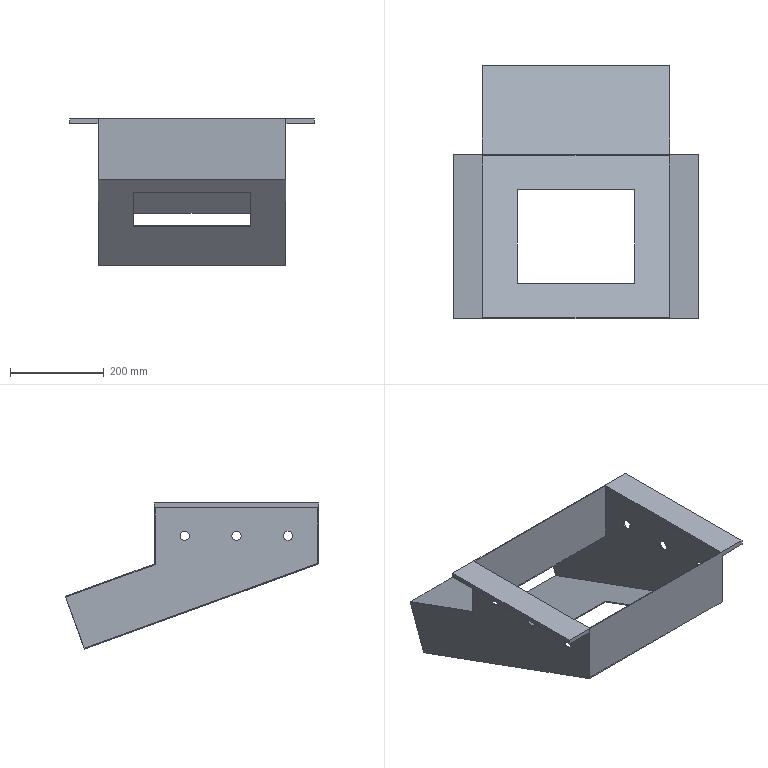Part | SolidWorks | features ICE 4, Extrusion 1, Shell 1 | 1 solid | 34 faces | box 520 x 538.979 x 311.271 mm | volume 1451807 mm3 | plane 22 | cylinder 12 | commonest cylinder face diameters 20 x12
STEP:
#1=CARTESIAN_POINT('',(198.,110.,50.));
#2=VERTEX_POINT('',#1);
#3=CARTESIAN_POINT('',(198.,110.,70.));
#4=VERTEX_POINT('',#3);
#5=CARTESIAN_POINT('',(198.,110.,60.));
#6=DIRECTION('',(-1.,0.,0.));
#7=DIRECTION('',(0.,0.,1.));
#8=AXIS2_PLACEMENT_3D('',#5,#6,#7);
#9=CIRCLE('',#8,10.);
#10=EDGE_CURVE('',#2,#4,#9,.T.);
#11=ORIENTED_EDGE('',*,*,#10,.T.);
#12=CARTESIAN_POINT('',(200.,110.,70.));
#13=VERTEX_POINT('',#12);
#14=CARTESIAN_POINT('',(-260.,110.,70.));
#15=DIRECTION('',(1.,0.,0.));
#16=VECTOR('',#15,1000.);
#17=LINE('',#14,#16);
#18=EDGE_CURVE('',#4,#13,#17,.T.);
#19=ORIENTED_EDGE('',*,*,#18,.T.);
#20=CARTESIAN_POINT('',(200.,110.,50.));
#21=VERTEX_POINT('',#20);
#22=CARTESIAN_POINT('',(200.,110.,60.));
#23=DIRECTION('',(1.,0.,0.));
#24=DIRECTION('',(0.,0.,-1.));
#25=AXIS2_PLACEMENT_3D('',#22,#23,#24);
#26=CIRCLE('',#25,10.);
#27=EDGE_CURVE('',#13,#21,#26,.T.);
#28=ORIENTED_EDGE('',*,*,#27,.T.);
#29=CARTESIAN_POINT('',(-260.,110.,50.));
#30=DIRECTION('',(1.,0.,0.));
#31=VECTOR('',#30,1000.);
#32=LINE('',#29,#31);
#33=EDGE_CURVE('',#2,#21,#32,.T.);
#34=ORIENTED_EDGE('',*,*,#33,.F.);
#35=EDGE_LOOP('',(#11,#19,#28,#34));
#36=FACE_OUTER_BOUND('',#35,.T.);
#37=CARTESIAN_POINT('',(-260.,110.,60.));
#38=DIRECTION('',(1.,0.,0.));
#39=DIRECTION('',(0.,0.,-1.));
#40=AXIS2_PLACEMENT_3D('',#37,#38,#39);
#41=CYLINDRICAL_SURFACE('',#40,10.);
#42=ADVANCED_FACE('',(#36),#41,.F.);
#43=CARTESIAN_POINT('',(198.,-110.,50.));
#44=VERTEX_POINT('',#43);
#45=CARTESIAN_POINT('',(198.,-110.,70.));
#46=VERTEX_POINT('',#45);
#47=CARTESIAN_POINT('',(198.,-110.,60.));
#48=DIRECTION('',(-1.,0.,0.));
#49=DIRECTION('',(0.,0.,1.));
#50=AXIS2_PLACEMENT_3D('',#47,#48,#49);
#51=CIRCLE('',#50,10.);
#52=EDGE_CURVE('',#44,#46,#51,.T.);
#53=ORIENTED_EDGE('',*,*,#52,.T.);
#54=CARTESIAN_POINT('',(200.,-110.,70.));
#55=VERTEX_POINT('',#54);
#56=CARTESIAN_POINT('',(-260.,-110.,70.));
#57=DIRECTION('',(1.,0.,0.));
#58=VECTOR('',#57,1000.);
#59=LINE('',#56,#58);
#60=EDGE_CURVE('',#46,#55,#59,.T.);
#61=ORIENTED_EDGE('',*,*,#60,.T.);
#62=CARTESIAN_POINT('',(200.,-110.,50.));
#63=VERTEX_POINT('',#62);
#64=CARTESIAN_POINT('',(200.,-110.,60.));
#65=DIRECTION('',(1.,0.,0.));
#66=DIRECTION('',(0.,0.,-1.));
#67=AXIS2_PLACEMENT_3D('',#64,#65,#66);
#68=CIRCLE('',#67,10.);
#69=EDGE_CURVE('',#55,#63,#68,.T.);
#70=ORIENTED_EDGE('',*,*,#69,.T.);
#71=CARTESIAN_POINT('',(-260.,-110.,50.));
#72=DIRECTION('',(1.,0.,0.));
#73=VECTOR('',#72,1000.);
#74=LINE('',#71,#73);
#75=EDGE_CURVE('',#44,#63,#74,.T.);
#76=ORIENTED_EDGE('',*,*,#75,.F.);
#77=EDGE_LOOP('',(#53,#61,#70,#76));
#78=FACE_OUTER_BOUND('',#77,.T.);
#79=CARTESIAN_POINT('',(-260.,-110.,60.));
#80=DIRECTION('',(1.,0.,0.));
#81=DIRECTION('',(0.,0.,-1.));
#82=AXIS2_PLACEMENT_3D('',#79,#80,#81);
#83=CYLINDRICAL_SURFACE('',#82,10.);
#84=ADVANCED_FACE('',(#78),#83,.F.);
#85=CARTESIAN_POINT('',(198.,0.,50.));
#86=VERTEX_POINT('',#85);
#87=CARTESIAN_POINT('',(198.,0.,70.));
#88=VERTEX_POINT('',#87);
#89=CARTESIAN_POINT('',(198.,0.,60.));
#90=DIRECTION('',(-1.,0.,0.));
#91=DIRECTION('',(0.,0.,1.));
#92=AXIS2_PLACEMENT_3D('',#89,#90,#91);
#93=CIRCLE('',#92,10.);
#94=EDGE_CURVE('',#86,#88,#93,.T.);
#95=ORIENTED_EDGE('',*,*,#94,.T.);
#96=CARTESIAN_POINT('',(200.,0.,70.));
#97=VERTEX_POINT('',#96);
#98=CARTESIAN_POINT('',(-260.,0.,70.));
#99=DIRECTION('',(1.,0.,0.));
#100=VECTOR('',#99,1000.);
#101=LINE('',#98,#100);
#102=EDGE_CURVE('',#88,#97,#101,.T.);
#103=ORIENTED_EDGE('',*,*,#102,.T.);
#104=CARTESIAN_POINT('',(200.,0.,50.));
#105=VERTEX_POINT('',#104);
#106=CARTESIAN_POINT('',(200.,0.,60.));
#107=DIRECTION('',(1.,0.,0.));
#108=DIRECTION('',(0.,0.,-1.));
#109=AXIS2_PLACEMENT_3D('',#106,#107,#108);
#110=CIRCLE('',#109,10.);
#111=EDGE_CURVE('',#97,#105,#110,.T.);
#112=ORIENTED_EDGE('',*,*,#111,.T.);
#113=CARTESIAN_POINT('',(-260.,0.,50.));
#114=DIRECTION('',(1.,0.,0.));
#115=VECTOR('',#114,1000.);
#116=LINE('',#113,#115);
#117=EDGE_CURVE('',#86,#105,#116,.T.);
#118=ORIENTED_EDGE('',*,*,#117,.F.);
#119=EDGE_LOOP('',(#95,#103,#112,#118));
#120=FACE_OUTER_BOUND('',#119,.T.);
#121=CARTESIAN_POINT('',(-260.,0.,60.));
#122=DIRECTION('',(1.,0.,0.));
#123=DIRECTION('',(0.,0.,-1.));
#124=AXIS2_PLACEMENT_3D('',#121,#122,#123);
#125=CYLINDRICAL_SURFACE('',#124,10.);
#126=ADVANCED_FACE('',(#120),#125,.F.);
#127=CARTESIAN_POINT('',(-200.,110.,70.));
#128=VERTEX_POINT('',#127);
#129=CARTESIAN_POINT('',(-200.,110.,50.));
#130=VERTEX_POINT('',#129);
#131=CARTESIAN_POINT('',(-200.,110.,60.));
#132=DIRECTION('',(1.,0.,0.));
#133=DIRECTION('',(0.,0.,-1.));
#134=AXIS2_PLACEMENT_3D('',#131,#132,#133);
#135=CIRCLE('',#134,10.);
#136=EDGE_CURVE('',#128,#130,#135,.T.);
#137=ORIENTED_EDGE('',*,*,#136,.F.);
#138=CARTESIAN_POINT('',(-198.,110.,70.));
#139=VERTEX_POINT('',#138);
#140=CARTESIAN_POINT('',(-260.,110.,70.));
#141=DIRECTION('',(1.,0.,0.));
#142=VECTOR('',#141,1000.);
#143=LINE('',#140,#142);
#144=EDGE_CURVE('',#128,#139,#143,.T.);
#145=ORIENTED_EDGE('',*,*,#144,.T.);
#146=CARTESIAN_POINT('',(-198.,110.,50.));
#147=VERTEX_POINT('',#146);
#148=CARTESIAN_POINT('',(-198.,110.,60.));
#149=DIRECTION('',(1.,0.,0.));
#150=DIRECTION('',(0.,0.,-1.));
#151=AXIS2_PLACEMENT_3D('',#148,#149,#150);
#152=CIRCLE('',#151,10.);
#153=EDGE_CURVE('',#139,#147,#152,.T.);
#154=ORIENTED_EDGE('',*,*,#153,.T.);
#155=CARTESIAN_POINT('',(-260.,110.,50.));
#156=DIRECTION('',(1.,0.,0.));
#157=VECTOR('',#156,1000.);
#158=LINE('',#155,#157);
#159=EDGE_CURVE('',#130,#147,#158,.T.);
#160=ORIENTED_EDGE('',*,*,#159,.F.);
#161=EDGE_LOOP('',(#137,#145,#154,#160));
#162=FACE_OUTER_BOUND('',#161,.T.);
#163=CARTESIAN_POINT('',(-260.,110.,60.));
#164=DIRECTION('',(1.,0.,0.));
#165=DIRECTION('',(0.,0.,-1.));
#166=AXIS2_PLACEMENT_3D('',#163,#164,#165);
#167=CYLINDRICAL_SURFACE('',#166,10.);
#168=ADVANCED_FACE('',(#162),#167,.F.);
#169=CARTESIAN_POINT('',(-200.,-110.,70.));
#170=VERTEX_POINT('',#169);
#171=CARTESIAN_POINT('',(-200.,-110.,50.));
#172=VERTEX_POINT('',#171);
#173=CARTESIAN_POINT('',(-200.,-110.,60.));
#174=DIRECTION('',(1.,0.,0.));
#175=DIRECTION('',(0.,0.,-1.));
#176=AXIS2_PLACEMENT_3D('',#173,#174,#175);
#177=CIRCLE('',#176,10.);
#178=EDGE_CURVE('',#170,#172,#177,.T.);
#179=ORIENTED_EDGE('',*,*,#178,.F.);
#180=CARTESIAN_POINT('',(-198.,-110.,70.));
#181=VERTEX_POINT('',#180);
#182=CARTESIAN_POINT('',(-260.,-110.,70.));
#183=DIRECTION('',(1.,0.,0.));
#184=VECTOR('',#183,1000.);
#185=LINE('',#182,#184);
#186=EDGE_CURVE('',#170,#181,#185,.T.);
#187=ORIENTED_EDGE('',*,*,#186,.T.);
#188=CARTESIAN_POINT('',(-198.,-110.,50.));
#189=VERTEX_POINT('',#188);
#190=CARTESIAN_POINT('',(-198.,-110.,60.));
#191=DIRECTION('',(1.,0.,0.));
#192=DIRECTION('',(0.,0.,-1.));
#193=AXIS2_PLACEMENT_3D('',#190,#191,#192);
#194=CIRCLE('',#193,10.);
#195=EDGE_CURVE('',#181,#189,#194,.T.);
#196=ORIENTED_EDGE('',*,*,#195,.T.);
#197=CARTESIAN_POINT('',(-260.,-110.,50.));
#198=DIRECTION('',(1.,0.,0.));
#199=VECTOR('',#198,1000.);
#200=LINE('',#197,#199);
#201=EDGE_CURVE('',#172,#189,#200,.T.);
#202=ORIENTED_EDGE('',*,*,#201,.F.);
#203=EDGE_LOOP('',(#179,#187,#196,#202));
#204=FACE_OUTER_BOUND('',#203,.T.);
#205=CARTESIAN_POINT('',(-260.,-110.,60.));
#206=DIRECTION('',(1.,0.,0.));
#207=DIRECTION('',(0.,0.,-1.));
#208=AXIS2_PLACEMENT_3D('',#205,#206,#207);
#209=CYLINDRICAL_SURFACE('',#208,10.);
#210=ADVANCED_FACE('',(#204),#209,.F.);
#211=CARTESIAN_POINT('',(-200.,0.,70.));
#212=VERTEX_POINT('',#211);
#213=CARTESIAN_POINT('',(-200.,0.,50.));
#214=VERTEX_POINT('',#213);
#215=CARTESIAN_POINT('',(-200.,0.,60.));
#216=DIRECTION('',(1.,0.,0.));
#217=DIRECTION('',(0.,0.,-1.));
#218=AXIS2_PLACEMENT_3D('',#215,#216,#217);
#219=CIRCLE('',#218,10.);
#220=EDGE_CURVE('',#212,#214,#219,.T.);
#221=ORIENTED_EDGE('',*,*,#220,.F.);
#222=CARTESIAN_POINT('',(-198.,0.,70.));
#223=VERTEX_POINT('',#222);
#224=CARTESIAN_POINT('',(-260.,0.,70.));
#225=DIRECTION('',(1.,0.,0.));
#226=VECTOR('',#225,1000.);
#227=LINE('',#224,#226);
#228=EDGE_CURVE('',#212,#223,#227,.T.);
#229=ORIENTED_EDGE('',*,*,#228,.T.);
#230=CARTESIAN_POINT('',(-198.,0.,50.));
#231=VERTEX_POINT('',#230);
#232=CARTESIAN_POINT('',(-198.,0.,60.));
#233=DIRECTION('',(1.,0.,0.));
#234=DIRECTION('',(0.,0.,-1.));
#235=AXIS2_PLACEMENT_3D('',#232,#233,#234);
#236=CIRCLE('',#235,10.);
#237=EDGE_CURVE('',#223,#231,#236,.T.);
#238=ORIENTED_EDGE('',*,*,#237,.T.);
#239=CARTESIAN_POINT('',(-260.,0.,50.));
#240=DIRECTION('',(1.,0.,0.));
#241=VECTOR('',#240,1000.);
#242=LINE('',#239,#241);
#243=EDGE_CURVE('',#214,#231,#242,.T.);
#244=ORIENTED_EDGE('',*,*,#243,.F.);
#245=EDGE_LOOP('',(#221,#229,#238,#244));
#246=FACE_OUTER_BOUND('',#245,.T.);
#247=CARTESIAN_POINT('',(-260.,0.,60.));
#248=DIRECTION('',(1.,0.,0.));
#249=DIRECTION('',(0.,0.,-1.));
#250=AXIS2_PLACEMENT_3D('',#247,#248,#249);
#251=CYLINDRICAL_SURFACE('',#250,10.);
#252=ADVANCED_FACE('',(#246),#251,.F.);
#253=CARTESIAN_POINT('',(-260.,-175.,130.));
#254=VERTEX_POINT('',#253);
#255=CARTESIAN_POINT('',(260.,-175.,130.));
#256=VERTEX_POINT('',#255);
#257=CARTESIAN_POINT('',(-200.,-175.,130.));
#258=DIRECTION('',(1.,0.,0.));
#259=VECTOR('',#258,1000.);
#260=LINE('',#257,#259);
#261=EDGE_CURVE('',#254,#256,#260,.T.);
#262=ORIENTED_EDGE('',*,*,#261,.T.);
#263=CARTESIAN_POINT('',(260.,175.,130.));
#264=VERTEX_POINT('',#263);
#265=CARTESIAN_POINT('',(260.,175.,130.));
#266=DIRECTION('',(0.,1.,0.));
#267=VECTOR('',#266,1000.);
#268=LINE('',#265,#267);
#269=EDGE_CURVE('',#256,#264,#268,.T.);
#270=ORIENTED_EDGE('',*,*,#269,.T.);
#271=CARTESIAN_POINT('',(-260.,175.,130.));
#272=VERTEX_POINT('',#271);
#273=CARTESIAN_POINT('',(-200.,175.,130.));
#274=DIRECTION('',(-1.,0.,0.));
#275=VECTOR('',#274,1000.);
#276=LINE('',#273,#275);
#277=EDGE_CURVE('',#264,#272,#276,.T.);
#278=ORIENTED_EDGE('',*,*,#277,.T.);
#279=CARTESIAN_POINT('',(-260.,175.,130.));
#280=DIRECTION('',(0.,-1.,0.));
#281=VECTOR('',#280,1000.);
#282=LINE('',#279,#281);
#283=EDGE_CURVE('',#272,#254,#282,.T.);
#284=ORIENTED_EDGE('',*,*,#283,.T.);
#285=EDGE_LOOP('',(#262,#270,#278,#284));
#286=FACE_OUTER_BOUND('',#285,.T.);
#287=CARTESIAN_POINT('',(198.,-173.,130.));
#288=VERTEX_POINT('',#287);
#289=CARTESIAN_POINT('',(198.,173.,130.));
#290=VERTEX_POINT('',#289);
#291=CARTESIAN_POINT('',(198.,0.,130.));
#292=DIRECTION('',(0.,1.,0.));
#293=VECTOR('',#292,1000.);
#294=LINE('',#291,#293);
#295=EDGE_CURVE('',#288,#290,#294,.T.);
#296=ORIENTED_EDGE('',*,*,#295,.F.);
#297=CARTESIAN_POINT('',(-198.,-173.,130.));
#298=VERTEX_POINT('',#297);
#299=CARTESIAN_POINT('',(0.,-173.,130.));
#300=DIRECTION('',(1.,0.,0.));
#301=VECTOR('',#300,1000.);
#302=LINE('',#299,#301);
#303=EDGE_CURVE('',#298,#288,#302,.T.);
#304=ORIENTED_EDGE('',*,*,#303,.F.);
#305=CARTESIAN_POINT('',(-198.,173.,130.));
#306=VERTEX_POINT('',#305);
#307=CARTESIAN_POINT('',(-198.,0.,130.));
#308=DIRECTION('',(0.,-1.,0.));
#309=VECTOR('',#308,1000.);
#310=LINE('',#307,#309);
#311=EDGE_CURVE('',#306,#298,#310,.T.);
#312=ORIENTED_EDGE('',*,*,#311,.F.);
#313=CARTESIAN_POINT('',(0.,173.,130.));
#314=DIRECTION('',(-1.,0.,0.));
#315=VECTOR('',#314,1000.);
#316=LINE('',#313,#315);
#317=EDGE_CURVE('',#290,#306,#316,.T.);
#318=ORIENTED_EDGE('',*,*,#317,.F.);
#319=EDGE_LOOP('',(#296,#304,#312,#318));
#320=FACE_BOUND('',#319,.T.);
#321=CARTESIAN_POINT('',(0.,0.,130.));
#322=DIRECTION('',(0.,0.,-1.));
#323=DIRECTION('',(-1.,0.,0.));
#324=AXIS2_PLACEMENT_3D('',#321,#322,#323);
#325=PLANE('',#324);
#326=ADVANCED_FACE('',(#286,#320),#325,.F.);
#327=CARTESIAN_POINT('',(200.,323.037,-181.271));
#328=VERTEX_POINT('',#327);
#329=CARTESIAN_POINT('',(200.,363.979,-68.783));
#330=VERTEX_POINT('',#329);
#331=CARTESIAN_POINT('',(200.,363.979,-68.783));
#332=DIRECTION('',(0.,0.342,0.9397));
#333=VECTOR('',#332,1000.);
#334=LINE('',#331,#333);
#335=EDGE_CURVE('',#328,#330,#334,.T.);
#336=ORIENTED_EDGE('',*,*,#335,.F.);
#337=CARTESIAN_POINT('',(-200.,323.037,-181.271));
#338=VERTEX_POINT('',#337);
#339=CARTESIAN_POINT('',(768.646,323.037,-181.271));
#340=DIRECTION('',(-1.,0.,0.));
#341=VECTOR('',#340,1000.);
#342=LINE('',#339,#341);
#343=EDGE_CURVE('',#328,#338,#342,.T.);
#344=ORIENTED_EDGE('',*,*,#343,.T.);
#345=CARTESIAN_POINT('',(-200.,363.979,-68.783));
#346=VERTEX_POINT('',#345);
#347=CARTESIAN_POINT('',(-200.,363.979,-68.783));
#348=DIRECTION('',(0.,-0.342,-0.9397));
#349=VECTOR('',#348,1000.);
#350=LINE('',#347,#349);
#351=EDGE_CURVE('',#346,#338,#350,.T.);
#352=ORIENTED_EDGE('',*,*,#351,.F.);
#353=CARTESIAN_POINT('',(768.646,363.979,-68.783));
#354=DIRECTION('',(-1.,0.,0.));
#355=VECTOR('',#354,1000.);
#356=LINE('',#353,#355);
#357=EDGE_CURVE('',#330,#346,#356,.T.);
#358=ORIENTED_EDGE('',*,*,#357,.F.);
#359=EDGE_LOOP('',(#336,#344,#352,#358));
#360=FACE_OUTER_BOUND('',#359,.T.);
#361=CARTESIAN_POINT('',(198.,323.721,-179.391));
#362=VERTEX_POINT('',#361);
#363=CARTESIAN_POINT('',(-198.,323.721,-179.391));
#364=VERTEX_POINT('',#363);
#365=CARTESIAN_POINT('',(768.646,323.721,-179.391));
#366=DIRECTION('',(-1.,0.,0.));
#367=VECTOR('',#366,1000.);
#368=LINE('',#365,#367);
#369=EDGE_CURVE('',#362,#364,#368,.T.);
#370=ORIENTED_EDGE('',*,*,#369,.F.);
#371=CARTESIAN_POINT('',(198.,363.295,-70.662));
#372=VERTEX_POINT('',#371);
#373=CARTESIAN_POINT('',(198.,363.979,-68.783));
#374=DIRECTION('',(0.,0.342,0.9397));
#375=VECTOR('',#374,1000.);
#376=LINE('',#373,#375);
#377=EDGE_CURVE('',#362,#372,#376,.T.);
#378=ORIENTED_EDGE('',*,*,#377,.T.);
#379=CARTESIAN_POINT('',(-198.,363.295,-70.662));
#380=VERTEX_POINT('',#379);
#381=CARTESIAN_POINT('',(768.646,363.295,-70.662));
#382=DIRECTION('',(-1.,0.,0.));
#383=VECTOR('',#382,1000.);
#384=LINE('',#381,#383);
#385=EDGE_CURVE('',#372,#380,#384,.T.);
#386=ORIENTED_EDGE('',*,*,#385,.T.);
#387=CARTESIAN_POINT('',(-198.,363.979,-68.783));
#388=DIRECTION('',(0.,-0.342,-0.9397));
#389=VECTOR('',#388,1000.);
#390=LINE('',#387,#389);
#391=EDGE_CURVE('',#380,#364,#390,.T.);
#392=ORIENTED_EDGE('',*,*,#391,.T.);
#393=EDGE_LOOP('',(#370,#378,#386,#392));
#394=FACE_BOUND('',#393,.T.);
#395=CARTESIAN_POINT('',(768.646,363.979,-68.783));
#396=DIRECTION('',(0.,0.9397,-0.342));
#397=DIRECTION('',(0.,0.342,0.9397));
#398=AXIS2_PLACEMENT_3D('',#395,#396,#397);
#399=PLANE('',#398);
#400=ADVANCED_FACE('',(#360,#394),#399,.T.);
#401=CARTESIAN_POINT('',(200.,110.,60.));
#402=DIRECTION('',(1.,0.,0.));
#403=DIRECTION('',(0.,0.,-1.));
#404=AXIS2_PLACEMENT_3D('',#401,#402,#403);
#405=CIRCLE('',#404,10.);
#406=EDGE_CURVE('',#21,#13,#405,.T.);
#407=ORIENTED_EDGE('',*,*,#406,.F.);
#408=ORIENTED_EDGE('',*,*,#27,.F.);
#409=EDGE_LOOP('',(#407,#408));
#410=FACE_BOUND('',#409,.T.);
#411=CARTESIAN_POINT('',(200.,-110.,60.));
#412=DIRECTION('',(1.,0.,0.));
#413=DIRECTION('',(0.,0.,-1.));
#414=AXIS2_PLACEMENT_3D('',#411,#412,#413);
#415=CIRCLE('',#414,10.);
#416=EDGE_CURVE('',#63,#55,#415,.T.);
#417=ORIENTED_EDGE('',*,*,#416,.F.);
#418=ORIENTED_EDGE('',*,*,#69,.F.);
#419=EDGE_LOOP('',(#417,#418));
#420=FACE_BOUND('',#419,.T.);
#421=CARTESIAN_POINT('',(200.,0.,60.));
#422=DIRECTION('',(1.,0.,0.));
#423=DIRECTION('',(0.,0.,-1.));
#424=AXIS2_PLACEMENT_3D('',#421,#422,#423);
#425=CIRCLE('',#424,10.);
#426=EDGE_CURVE('',#105,#97,#425,.T.);
#427=ORIENTED_EDGE('',*,*,#426,.F.);
#428=ORIENTED_EDGE('',*,*,#111,.F.);
#429=EDGE_LOOP('',(#427,#428));
#430=FACE_BOUND('',#429,.T.);
#431=CARTESIAN_POINT('',(200.,175.,120.));
#432=VERTEX_POINT('',#431);
#433=CARTESIAN_POINT('',(200.,175.,0.));
#434=VERTEX_POINT('',#433);
#435=CARTESIAN_POINT('',(200.,175.,130.));
#436=DIRECTION('',(0.,0.,-1.));
#437=VECTOR('',#436,1000.);
#438=LINE('',#435,#437);
#439=EDGE_CURVE('',#432,#434,#438,.T.);
#440=ORIENTED_EDGE('',*,*,#439,.F.);
#441=CARTESIAN_POINT('',(200.,-175.,120.));
#442=VERTEX_POINT('',#441);
#443=CARTESIAN_POINT('',(200.,175.,120.));
#444=DIRECTION('',(0.,-1.,0.));
#445=VECTOR('',#444,1000.);
#446=LINE('',#443,#445);
#447=EDGE_CURVE('',#432,#442,#446,.T.);
#448=ORIENTED_EDGE('',*,*,#447,.T.);
#449=CARTESIAN_POINT('',(200.,-175.,0.));
#450=VERTEX_POINT('',#449);
#451=CARTESIAN_POINT('',(200.,-175.,130.));
#452=DIRECTION('',(0.,0.,-1.));
#453=VECTOR('',#452,1000.);
#454=LINE('',#451,#453);
#455=EDGE_CURVE('',#442,#450,#454,.T.);
#456=ORIENTED_EDGE('',*,*,#455,.T.);
#457=CARTESIAN_POINT('',(200.,323.037,-181.271));
#458=DIRECTION('',(0.,0.9397,-0.342));
#459=VECTOR('',#458,1000.);
#460=LINE('',#457,#459);
#461=EDGE_CURVE('',#450,#328,#460,.T.);
#462=ORIENTED_EDGE('',*,*,#461,.T.);
#463=ORIENTED_EDGE('',*,*,#335,.T.);
#464=CARTESIAN_POINT('',(200.,175.,0.));
#465=DIRECTION('',(0.,-0.9397,0.342));
#466=VECTOR('',#465,1000.);
#467=LINE('',#464,#466);
#468=EDGE_CURVE('',#330,#434,#467,.T.);
#469=ORIENTED_EDGE('',*,*,#468,.T.);
#470=EDGE_LOOP('',(#440,#448,#456,#462,#463,#469));
#471=FACE_OUTER_BOUND('',#470,.T.);
#472=CARTESIAN_POINT('',(200.,-175.,130.));
#473=DIRECTION('',(-1.,0.,0.));
#474=DIRECTION('',(0.,0.,1.));
#475=AXIS2_PLACEMENT_3D('',#472,#473,#474);
#476=PLANE('',#475);
#477=ADVANCED_FACE('',(#410,#420,#430,#471),#476,.F.);
#478=CARTESIAN_POINT('',(-200.,175.,0.));
#479=VERTEX_POINT('',#478);
#480=CARTESIAN_POINT('',(-200.,175.,0.));
#481=DIRECTION('',(-1.,0.,0.));
#482=VECTOR('',#481,1000.);
#483=LINE('',#480,#482);
#484=EDGE_CURVE('',#434,#479,#483,.T.);
#485=ORIENTED_EDGE('',*,*,#484,.T.);
#486=CARTESIAN_POINT('',(-200.,175.,120.));
#487=VERTEX_POINT('',#486);
#488=CARTESIAN_POINT('',(-200.,175.,130.));
#489=DIRECTION('',(0.,0.,-1.));
#490=VECTOR('',#489,1000.);
#491=LINE('',#488,#490);
#492=EDGE_CURVE('',#487,#479,#491,.T.);
#493=ORIENTED_EDGE('',*,*,#492,.F.);
#494=CARTESIAN_POINT('',(-260.,175.,120.));
#495=VERTEX_POINT('',#494);
#496=CARTESIAN_POINT('',(-200.,175.,120.));
#497=DIRECTION('',(-1.,0.,0.));
#498=VECTOR('',#497,1000.);
#499=LINE('',#496,#498);
#500=EDGE_CURVE('',#487,#495,#499,.T.);
#501=ORIENTED_EDGE('',*,*,#500,.T.);
#502=CARTESIAN_POINT('',(-260.,175.,120.));
#503=DIRECTION('',(0.,0.,1.));
#504=VECTOR('',#503,1000.);
#505=LINE('',#502,#504);
#506=EDGE_CURVE('',#495,#272,#505,.T.);
#507=ORIENTED_EDGE('',*,*,#506,.T.);
#508=ORIENTED_EDGE('',*,*,#277,.F.);
#509=CARTESIAN_POINT('',(260.,175.,120.));
#510=VERTEX_POINT('',#509);
#511=CARTESIAN_POINT('',(260.,175.,120.));
#512=DIRECTION('',(0.,0.,1.));
#513=VECTOR('',#512,1000.);
#514=LINE('',#511,#513);
#515=EDGE_CURVE('',#510,#264,#514,.T.);
#516=ORIENTED_EDGE('',*,*,#515,.F.);
#517=CARTESIAN_POINT('',(200.,175.,120.));
#518=DIRECTION('',(-1.,0.,0.));
#519=VECTOR('',#518,1000.);
#520=LINE('',#517,#519);
#521=EDGE_CURVE('',#510,#432,#520,.T.);
#522=ORIENTED_EDGE('',*,*,#521,.T.);
#523=ORIENTED_EDGE('',*,*,#439,.T.);
#524=EDGE_LOOP('',(#485,#493,#501,#507,#508,#516,#522,#523));
#525=FACE_OUTER_BOUND('',#524,.T.);
#526=CARTESIAN_POINT('',(-200.,175.,130.));
#527=DIRECTION('',(0.,-1.,0.));
#528=DIRECTION('',(0.,0.,-1.));
#529=AXIS2_PLACEMENT_3D('',#526,#527,#528);
#530=PLANE('',#529);
#531=ADVANCED_FACE('',(#525),#530,.F.);
#532=CARTESIAN_POINT('',(-200.,110.,60.));
#533=DIRECTION('',(1.,0.,0.));
#534=DIRECTION('',(0.,0.,-1.));
#535=AXIS2_PLACEMENT_3D('',#532,#533,#534);
#536=CIRCLE('',#535,10.);
#537=EDGE_CURVE('',#130,#128,#536,.T.);
#538=ORIENTED_EDGE('',*,*,#537,.T.);
#539=ORIENTED_EDGE('',*,*,#136,.T.);
#540=EDGE_LOOP('',(#538,#539));
#541=FACE_BOUND('',#540,.T.);
#542=CARTESIAN_POINT('',(-200.,-110.,60.));
#543=DIRECTION('',(1.,0.,0.));
#544=DIRECTION('',(0.,0.,-1.));
#545=AXIS2_PLACEMENT_3D('',#542,#543,#544);
#546=CIRCLE('',#545,10.);
#547=EDGE_CURVE('',#172,#170,#546,.T.);
#548=ORIENTED_EDGE('',*,*,#547,.T.);
#549=ORIENTED_EDGE('',*,*,#178,.T.);
#550=EDGE_LOOP('',(#548,#549));
#551=FACE_BOUND('',#550,.T.);
#552=CARTESIAN_POINT('',(-200.,0.,60.));
#553=DIRECTION('',(1.,0.,0.));
#554=DIRECTION('',(0.,0.,-1.));
#555=AXIS2_PLACEMENT_3D('',#552,#553,#554);
#556=CIRCLE('',#555,10.);
#557=EDGE_CURVE('',#214,#212,#556,.T.);
#558=ORIENTED_EDGE('',*,*,#557,.T.);
#559=ORIENTED_EDGE('',*,*,#220,.T.);
#560=EDGE_LOOP('',(#558,#559));
#561=FACE_BOUND('',#560,.T.);
#562=CARTESIAN_POINT('',(-200.,-175.,120.));
#563=VERTEX_POINT('',#562);
#564=CARTESIAN_POINT('',(-200.,-175.,0.));
#565=VERTEX_POINT('',#564);
#566=CARTESIAN_POINT('',(-200.,-175.,130.));
#567=DIRECTION('',(0.,0.,-1.));
#568=VECTOR('',#567,1000.);
#569=LINE('',#566,#568);
#570=EDGE_CURVE('',#563,#565,#569,.T.);
#571=ORIENTED_EDGE('',*,*,#570,.F.);
#572=CARTESIAN_POINT('',(-200.,175.,120.));
#573=DIRECTION('',(0.,1.,0.));
#574=VECTOR('',#573,1000.);
#575=LINE('',#572,#574);
#576=EDGE_CURVE('',#563,#487,#575,.T.);
#577=ORIENTED_EDGE('',*,*,#576,.T.);
#578=ORIENTED_EDGE('',*,*,#492,.T.);
#579=CARTESIAN_POINT('',(-200.,175.,0.));
#580=DIRECTION('',(0.,0.9397,-0.342));
#581=VECTOR('',#580,1000.);
#582=LINE('',#579,#581);
#583=EDGE_CURVE('',#479,#346,#582,.T.);
#584=ORIENTED_EDGE('',*,*,#583,.T.);
#585=ORIENTED_EDGE('',*,*,#351,.T.);
#586=CARTESIAN_POINT('',(-200.,323.037,-181.271));
#587=DIRECTION('',(0.,-0.9397,0.342));
#588=VECTOR('',#587,1000.);
#589=LINE('',#586,#588);
#590=EDGE_CURVE('',#338,#565,#589,.T.);
#591=ORIENTED_EDGE('',*,*,#590,.T.);
#592=EDGE_LOOP('',(#571,#577,#578,#584,#585,#591));
#593=FACE_OUTER_BOUND('',#592,.T.);
#594=CARTESIAN_POINT('',(-200.,-175.,130.));
#595=DIRECTION('',(1.,0.,0.));
#596=DIRECTION('',(0.,0.,-1.));
#597=AXIS2_PLACEMENT_3D('',#594,#595,#596);
#598=PLANE('',#597);
#599=ADVANCED_FACE('',(#541,#551,#561,#593),#598,.F.);
#600=CARTESIAN_POINT('',(-200.,-175.,0.));
#601=DIRECTION('',(1.,0.,0.));
#602=VECTOR('',#601,1000.);
#603=LINE('',#600,#602);
#604=EDGE_CURVE('',#565,#450,#603,.T.);
#605=ORIENTED_EDGE('',*,*,#604,.T.);
#606=ORIENTED_EDGE('',*,*,#455,.F.);
#607=CARTESIAN_POINT('',(260.,-175.,120.));
#608=VERTEX_POINT('',#607);
#609=CARTESIAN_POINT('',(200.,-175.,120.));
#610=DIRECTION('',(1.,0.,0.));
#611=VECTOR('',#610,1000.);
#612=LINE('',#609,#611);
#613=EDGE_CURVE('',#442,#608,#612,.T.);
#614=ORIENTED_EDGE('',*,*,#613,.T.);
#615=CARTESIAN_POINT('',(260.,-175.,120.));
#616=DIRECTION('',(0.,0.,1.));
#617=VECTOR('',#616,1000.);
#618=LINE('',#615,#617);
#619=EDGE_CURVE('',#608,#256,#618,.T.);
#620=ORIENTED_EDGE('',*,*,#619,.T.);
#621=ORIENTED_EDGE('',*,*,#261,.F.);
#622=CARTESIAN_POINT('',(-260.,-175.,120.));
#623=VERTEX_POINT('',#622);
#624=CARTESIAN_POINT('',(-260.,-175.,120.));
#625=DIRECTION('',(0.,0.,1.));
#626=VECTOR('',#625,1000.);
#627=LINE('',#624,#626);
#628=EDGE_CURVE('',#623,#254,#627,.T.);
#629=ORIENTED_EDGE('',*,*,#628,.F.);
#630=CARTESIAN_POINT('',(-200.,-175.,120.));
#631=DIRECTION('',(1.,0.,0.));
#632=VECTOR('',#631,1000.);
#633=LINE('',#630,#632);
#634=EDGE_CURVE('',#623,#563,#633,.T.);
#635=ORIENTED_EDGE('',*,*,#634,.T.);
#636=ORIENTED_EDGE('',*,*,#570,.T.);
#637=EDGE_LOOP('',(#605,#606,#614,#620,#621,#629,#635,#636));
#638=FACE_OUTER_BOUND('',#637,.T.);
#639=CARTESIAN_POINT('',(-200.,-175.,130.));
#640=DIRECTION('',(0.,1.,0.));
#641=DIRECTION('',(0.,0.,1.));
#642=AXIS2_PLACEMENT_3D('',#639,#640,#641);
#643=PLANE('',#642);
#644=ADVANCED_FACE('',(#638),#643,.F.);
#645=CARTESIAN_POINT('',(125.,100.,-100.092));
#646=VERTEX_POINT('',#645);
#647=CARTESIAN_POINT('',(125.,-100.,-27.298));
#648=VERTEX_POINT('',#647);
#649=CARTESIAN_POINT('',(125.,323.037,-181.271));
#650=DIRECTION('',(0.,-0.9397,0.342));
#651=VECTOR('',#650,1000.);
#652=LINE('',#649,#651);
#653=EDGE_CURVE('',#646,#648,#652,.T.);
#654=ORIENTED_EDGE('',*,*,#653,.F.);
#655=CARTESIAN_POINT('',(-125.,100.,-100.092));
#656=VERTEX_POINT('',#655);
#657=CARTESIAN_POINT('',(768.646,100.,-100.092));
#658=DIRECTION('',(1.,0.,0.));
#659=VECTOR('',#658,1000.);
#660=LINE('',#657,#659);
#661=EDGE_CURVE('',#656,#646,#660,.T.);
#662=ORIENTED_EDGE('',*,*,#661,.F.);
#663=CARTESIAN_POINT('',(-125.,-100.,-27.298));
#664=VERTEX_POINT('',#663);
#665=CARTESIAN_POINT('',(-125.,323.037,-181.271));
#666=DIRECTION('',(0.,0.9397,-0.342));
#667=VECTOR('',#666,1000.);
#668=LINE('',#665,#667);
#669=EDGE_CURVE('',#664,#656,#668,.T.);
#670=ORIENTED_EDGE('',*,*,#669,.F.);
#671=CARTESIAN_POINT('',(768.646,-100.,-27.298));
#672=DIRECTION('',(-1.,0.,0.));
#673=VECTOR('',#672,1000.);
#674=LINE('',#671,#673);
#675=EDGE_CURVE('',#648,#664,#674,.T.);
#676=ORIENTED_EDGE('',*,*,#675,.F.);
#677=EDGE_LOOP('',(#654,#662,#670,#676));
#678=FACE_BOUND('',#677,.T.);
#679=ORIENTED_EDGE('',*,*,#461,.F.);
#680=ORIENTED_EDGE('',*,*,#604,.F.);
#681=ORIENTED_EDGE('',*,*,#590,.F.);
#682=ORIENTED_EDGE('',*,*,#343,.F.);
#683=EDGE_LOOP('',(#679,#680,#681,#682));
#684=FACE_OUTER_BOUND('',#683,.T.);
#685=CARTESIAN_POINT('',(768.646,323.037,-181.271));
#686=DIRECTION('',(0.,-0.342,-0.9397));
#687=DIRECTION('',(0.,0.9397,-0.342));
#688=AXIS2_PLACEMENT_3D('',#685,#686,#687);
#689=PLANE('',#688);
#690=ADVANCED_FACE('',(#678,#684),#689,.T.);
#691=ORIENTED_EDGE('',*,*,#468,.F.);
#692=ORIENTED_EDGE('',*,*,#357,.T.);
#693=ORIENTED_EDGE('',*,*,#583,.F.);
#694=ORIENTED_EDGE('',*,*,#484,.F.);
#695=EDGE_LOOP('',(#691,#692,#693,#694));
#696=FACE_OUTER_BOUND('',#695,.T.);
#697=CARTESIAN_POINT('',(768.646,175.,0.));
#698=DIRECTION('',(0.,0.342,0.9397));
#699=DIRECTION('',(0.,-0.9397,0.342));
#700=AXIS2_PLACEMENT_3D('',#697,#698,#699);
#701=PLANE('',#700);
#702=ADVANCED_FACE('',(#696),#701,.T.);
#703=ORIENTED_EDGE('',*,*,#10,.F.);
#704=CARTESIAN_POINT('',(198.,110.,60.));
#705=DIRECTION('',(-1.,0.,0.));
#706=DIRECTION('',(0.,0.,1.));
#707=AXIS2_PLACEMENT_3D('',#704,#705,#706);
#708=CIRCLE('',#707,10.);
#709=EDGE_CURVE('',#4,#2,#708,.T.);
#710=ORIENTED_EDGE('',*,*,#709,.F.);
#711=EDGE_LOOP('',(#703,#710));
#712=FACE_BOUND('',#711,.T.);
#713=ORIENTED_EDGE('',*,*,#52,.F.);
#714=CARTESIAN_POINT('',(198.,-110.,60.));
#715=DIRECTION('',(-1.,0.,0.));
#716=DIRECTION('',(0.,0.,1.));
#717=AXIS2_PLACEMENT_3D('',#714,#715,#716);
#718=CIRCLE('',#717,10.);
#719=EDGE_CURVE('',#46,#44,#718,.T.);
#720=ORIENTED_EDGE('',*,*,#719,.F.);
#721=EDGE_LOOP('',(#713,#720));
#722=FACE_BOUND('',#721,.T.);
#723=ORIENTED_EDGE('',*,*,#94,.F.);
#724=CARTESIAN_POINT('',(198.,0.,60.));
#725=DIRECTION('',(-1.,0.,0.));
#726=DIRECTION('',(0.,0.,1.));
#727=AXIS2_PLACEMENT_3D('',#724,#725,#726);
#728=CIRCLE('',#727,10.);
#729=EDGE_CURVE('',#88,#86,#728,.T.);
#730=ORIENTED_EDGE('',*,*,#729,.F.);
#731=EDGE_LOOP('',(#723,#730));
#732=FACE_BOUND('',#731,.T.);
#733=CARTESIAN_POINT('',(198.,-173.,1.4));
#734=VERTEX_POINT('',#733);
#735=CARTESIAN_POINT('',(198.,-173.,130.));
#736=DIRECTION('',(0.,0.,-1.));
#737=VECTOR('',#736,1000.);
#738=LINE('',#735,#737);
#739=EDGE_CURVE('',#288,#734,#738,.T.);
#740=ORIENTED_EDGE('',*,*,#739,.F.);
#741=ORIENTED_EDGE('',*,*,#295,.T.);
#742=CARTESIAN_POINT('',(198.,173.,-1.4));
#743=VERTEX_POINT('',#742);
#744=CARTESIAN_POINT('',(198.,173.,130.));
#745=DIRECTION('',(0.,0.,-1.));
#746=VECTOR('',#745,1000.);
#747=LINE('',#744,#746);
#748=EDGE_CURVE('',#290,#743,#747,.T.);
#749=ORIENTED_EDGE('',*,*,#748,.T.);
#750=CARTESIAN_POINT('',(198.,174.316,-1.879));
#751=DIRECTION('',(0.,-0.9397,0.342));
#752=VECTOR('',#751,1000.);
#753=LINE('',#750,#752);
#754=EDGE_CURVE('',#372,#743,#753,.T.);
#755=ORIENTED_EDGE('',*,*,#754,.F.);
#756=ORIENTED_EDGE('',*,*,#377,.F.);
#757=CARTESIAN_POINT('',(198.,323.721,-179.391));
#758=DIRECTION('',(0.,0.9397,-0.342));
#759=VECTOR('',#758,1000.);
#760=LINE('',#757,#759);
#761=EDGE_CURVE('',#734,#362,#760,.T.);
#762=ORIENTED_EDGE('',*,*,#761,.F.);
#763=EDGE_LOOP('',(#740,#741,#749,#755,#756,#762));
#764=FACE_OUTER_BOUND('',#763,.T.);
#765=CARTESIAN_POINT('',(198.,-175.,130.));
#766=DIRECTION('',(-1.,0.,0.));
#767=DIRECTION('',(0.,0.,1.));
#768=AXIS2_PLACEMENT_3D('',#765,#766,#767);
#769=PLANE('',#768);
#770=ADVANCED_FACE('',(#712,#722,#732,#764),#769,.T.);
#771=CARTESIAN_POINT('',(-198.,173.,-1.4));
#772=VERTEX_POINT('',#771);
#773=CARTESIAN_POINT('',(-200.,173.,-1.4));
#774=DIRECTION('',(-1.,0.,0.));
#775=VECTOR('',#774,1000.);
#776=LINE('',#773,#775);
#777=EDGE_CURVE('',#743,#772,#776,.T.);
#778=ORIENTED_EDGE('',*,*,#777,.F.);
#779=ORIENTED_EDGE('',*,*,#748,.F.);
#780=ORIENTED_EDGE('',*,*,#317,.T.);
#781=CARTESIAN_POINT('',(-198.,173.,130.));
#782=DIRECTION('',(0.,0.,-1.));
#783=VECTOR('',#782,1000.);
#784=LINE('',#781,#783);
#785=EDGE_CURVE('',#306,#772,#784,.T.);
#786=ORIENTED_EDGE('',*,*,#785,.T.);
#787=EDGE_LOOP('',(#778,#779,#780,#786));
#788=FACE_OUTER_BOUND('',#787,.T.);
#789=CARTESIAN_POINT('',(-200.,173.,130.));
#790=DIRECTION('',(0.,-1.,0.));
#791=DIRECTION('',(0.,0.,-1.));
#792=AXIS2_PLACEMENT_3D('',#789,#790,#791);
#793=PLANE('',#792);
#794=ADVANCED_FACE('',(#788),#793,.T.);
#795=CARTESIAN_POINT('',(-198.,110.,60.));
#796=DIRECTION('',(1.,0.,0.));
#797=DIRECTION('',(0.,0.,-1.));
#798=AXIS2_PLACEMENT_3D('',#795,#796,#797);
#799=CIRCLE('',#798,10.);
#800=EDGE_CURVE('',#147,#139,#799,.T.);
#801=ORIENTED_EDGE('',*,*,#800,.F.);
#802=ORIENTED_EDGE('',*,*,#153,.F.);
#803=EDGE_LOOP('',(#801,#802));
#804=FACE_BOUND('',#803,.T.);
#805=CARTESIAN_POINT('',(-198.,-110.,60.));
#806=DIRECTION('',(1.,0.,0.));
#807=DIRECTION('',(0.,0.,-1.));
#808=AXIS2_PLACEMENT_3D('',#805,#806,#807);
#809=CIRCLE('',#808,10.);
#810=EDGE_CURVE('',#189,#181,#809,.T.);
#811=ORIENTED_EDGE('',*,*,#810,.F.);
#812=ORIENTED_EDGE('',*,*,#195,.F.);
#813=EDGE_LOOP('',(#811,#812));
#814=FACE_BOUND('',#813,.T.);
#815=CARTESIAN_POINT('',(-198.,0.,60.));
#816=DIRECTION('',(1.,0.,0.));
#817=DIRECTION('',(0.,0.,-1.));
#818=AXIS2_PLACEMENT_3D('',#815,#816,#817);
#819=CIRCLE('',#818,10.);
#820=EDGE_CURVE('',#231,#223,#819,.T.);
#821=ORIENTED_EDGE('',*,*,#820,.F.);
#822=ORIENTED_EDGE('',*,*,#237,.F.);
#823=EDGE_LOOP('',(#821,#822));
#824=FACE_BOUND('',#823,.T.);
#825=ORIENTED_EDGE('',*,*,#785,.F.);
#826=ORIENTED_EDGE('',*,*,#311,.T.);
#827=CARTESIAN_POINT('',(-198.,-173.,1.4));
#828=VERTEX_POINT('',#827);
#829=CARTESIAN_POINT('',(-198.,-173.,130.));
#830=DIRECTION('',(0.,0.,-1.));
#831=VECTOR('',#830,1000.);
#832=LINE('',#829,#831);
#833=EDGE_CURVE('',#298,#828,#832,.T.);
#834=ORIENTED_EDGE('',*,*,#833,.T.);
#835=CARTESIAN_POINT('',(-198.,323.721,-179.391));
#836=DIRECTION('',(0.,-0.9397,0.342));
#837=VECTOR('',#836,1000.);
#838=LINE('',#835,#837);
#839=EDGE_CURVE('',#364,#828,#838,.T.);
#840=ORIENTED_EDGE('',*,*,#839,.F.);
#841=ORIENTED_EDGE('',*,*,#391,.F.);
#842=CARTESIAN_POINT('',(-198.,174.316,-1.879));
#843=DIRECTION('',(0.,0.9397,-0.342));
#844=VECTOR('',#843,1000.);
#845=LINE('',#842,#844);
#846=EDGE_CURVE('',#772,#380,#845,.T.);
#847=ORIENTED_EDGE('',*,*,#846,.F.);
#848=EDGE_LOOP('',(#825,#826,#834,#840,#841,#847));
#849=FACE_OUTER_BOUND('',#848,.T.);
#850=CARTESIAN_POINT('',(-198.,-175.,130.));
#851=DIRECTION('',(1.,0.,0.));
#852=DIRECTION('',(0.,0.,-1.));
#853=AXIS2_PLACEMENT_3D('',#850,#851,#852);
#854=PLANE('',#853);
#855=ADVANCED_FACE('',(#804,#814,#824,#849),#854,.T.);
#856=CARTESIAN_POINT('',(768.646,-173.,1.4));
#857=DIRECTION('',(1.,0.,0.));
#858=VECTOR('',#857,1000.);
#859=LINE('',#856,#858);
#860=EDGE_CURVE('',#828,#734,#859,.T.);
#861=ORIENTED_EDGE('',*,*,#860,.F.);
#862=ORIENTED_EDGE('',*,*,#833,.F.);
#863=ORIENTED_EDGE('',*,*,#303,.T.);
#864=ORIENTED_EDGE('',*,*,#739,.T.);
#865=EDGE_LOOP('',(#861,#862,#863,#864));
#866=FACE_OUTER_BOUND('',#865,.T.);
#867=CARTESIAN_POINT('',(-200.,-173.,130.));
#868=DIRECTION('',(0.,1.,0.));
#869=DIRECTION('',(0.,0.,1.));
#870=AXIS2_PLACEMENT_3D('',#867,#868,#869);
#871=PLANE('',#870);
#872=ADVANCED_FACE('',(#866),#871,.T.);
#873=CARTESIAN_POINT('',(-125.,100.,-97.963));
#874=VERTEX_POINT('',#873);
#875=CARTESIAN_POINT('',(125.,100.,-97.963));
#876=VERTEX_POINT('',#875);
#877=CARTESIAN_POINT('',(768.646,100.,-97.963));
#878=DIRECTION('',(1.,0.,0.));
#879=VECTOR('',#878,1000.);
#880=LINE('',#877,#879);
#881=EDGE_CURVE('',#874,#876,#880,.T.);
#882=ORIENTED_EDGE('',*,*,#881,.T.);
#883=CARTESIAN_POINT('',(125.,-100.,-25.169));
#884=VERTEX_POINT('',#883);
#885=CARTESIAN_POINT('',(125.,323.721,-179.391));
#886=DIRECTION('',(0.,-0.9397,0.342));
#887=VECTOR('',#886,1000.);
#888=LINE('',#885,#887);
#889=EDGE_CURVE('',#876,#884,#888,.T.);
#890=ORIENTED_EDGE('',*,*,#889,.T.);
#891=CARTESIAN_POINT('',(-125.,-100.,-25.169));
#892=VERTEX_POINT('',#891);
#893=CARTESIAN_POINT('',(768.646,-100.,-25.169));
#894=DIRECTION('',(-1.,0.,0.));
#895=VECTOR('',#894,1000.);
#896=LINE('',#893,#895);
#897=EDGE_CURVE('',#884,#892,#896,.T.);
#898=ORIENTED_EDGE('',*,*,#897,.T.);
#899=CARTESIAN_POINT('',(-125.,323.721,-179.391));
#900=DIRECTION('',(0.,0.9397,-0.342));
#901=VECTOR('',#900,1000.);
#902=LINE('',#899,#901);
#903=EDGE_CURVE('',#892,#874,#902,.T.);
#904=ORIENTED_EDGE('',*,*,#903,.T.);
#905=EDGE_LOOP('',(#882,#890,#898,#904));
#906=FACE_BOUND('',#905,.T.);
#907=ORIENTED_EDGE('',*,*,#761,.T.);
#908=ORIENTED_EDGE('',*,*,#369,.T.);
#909=ORIENTED_EDGE('',*,*,#839,.T.);
#910=ORIENTED_EDGE('',*,*,#860,.T.);
#911=EDGE_LOOP('',(#907,#908,#909,#910));
#912=FACE_OUTER_BOUND('',#911,.T.);
#913=CARTESIAN_POINT('',(768.646,323.721,-179.391));
#914=DIRECTION('',(0.,-0.342,-0.9397));
#915=DIRECTION('',(0.,0.9397,-0.342));
#916=AXIS2_PLACEMENT_3D('',#913,#914,#915);
#917=PLANE('',#916);
#918=ADVANCED_FACE('',(#906,#912),#917,.F.);
#919=ORIENTED_EDGE('',*,*,#754,.T.);
#920=ORIENTED_EDGE('',*,*,#777,.T.);
#921=ORIENTED_EDGE('',*,*,#846,.T.);
#922=ORIENTED_EDGE('',*,*,#385,.F.);
#923=EDGE_LOOP('',(#919,#920,#921,#922));
#924=FACE_OUTER_BOUND('',#923,.T.);
#925=CARTESIAN_POINT('',(768.646,174.316,-1.879));
#926=DIRECTION('',(0.,0.342,0.9397));
#927=DIRECTION('',(0.,-0.9397,0.342));
#928=AXIS2_PLACEMENT_3D('',#925,#926,#927);
#929=PLANE('',#928);
#930=ADVANCED_FACE('',(#924),#929,.F.);
#931=ORIENTED_EDGE('',*,*,#283,.F.);
#932=ORIENTED_EDGE('',*,*,#506,.F.);
#933=CARTESIAN_POINT('',(-260.,175.,120.));
#934=DIRECTION('',(0.,-1.,0.));
#935=VECTOR('',#934,1000.);
#936=LINE('',#933,#935);
#937=EDGE_CURVE('',#495,#623,#936,.T.);
#938=ORIENTED_EDGE('',*,*,#937,.T.);
#939=ORIENTED_EDGE('',*,*,#628,.T.);
#940=EDGE_LOOP('',(#931,#932,#938,#939));
#941=FACE_OUTER_BOUND('',#940,.T.);
#942=CARTESIAN_POINT('',(-260.,175.,120.));
#943=DIRECTION('',(-1.,0.,0.));
#944=DIRECTION('',(0.,-1.,0.));
#945=AXIS2_PLACEMENT_3D('',#942,#943,#944);
#946=PLANE('',#945);
#947=ADVANCED_FACE('',(#941),#946,.T.);
#948=ORIENTED_EDGE('',*,*,#576,.F.);
#949=ORIENTED_EDGE('',*,*,#634,.F.);
#950=ORIENTED_EDGE('',*,*,#937,.F.);
#951=ORIENTED_EDGE('',*,*,#500,.F.);
#952=EDGE_LOOP('',(#948,#949,#950,#951));
#953=FACE_OUTER_BOUND('',#952,.T.);
#954=CARTESIAN_POINT('',(0.,0.,120.));
#955=DIRECTION('',(0.,0.,-1.));
#956=DIRECTION('',(-1.,0.,0.));
#957=AXIS2_PLACEMENT_3D('',#954,#955,#956);
#958=PLANE('',#957);
#959=ADVANCED_FACE('',(#953),#958,.T.);
#960=ORIENTED_EDGE('',*,*,#269,.F.);
#961=ORIENTED_EDGE('',*,*,#619,.F.);
#962=CARTESIAN_POINT('',(260.,175.,120.));
#963=DIRECTION('',(0.,1.,0.));
#964=VECTOR('',#963,1000.);
#965=LINE('',#962,#964);
#966=EDGE_CURVE('',#608,#510,#965,.T.);
#967=ORIENTED_EDGE('',*,*,#966,.T.);
#968=ORIENTED_EDGE('',*,*,#515,.T.);
#969=EDGE_LOOP('',(#960,#961,#967,#968));
#970=FACE_OUTER_BOUND('',#969,.T.);
#971=CARTESIAN_POINT('',(260.,175.,120.));
#972=DIRECTION('',(1.,0.,0.));
#973=DIRECTION('',(0.,1.,0.));
#974=AXIS2_PLACEMENT_3D('',#971,#972,#973);
#975=PLANE('',#974);
#976=ADVANCED_FACE('',(#970),#975,.T.);
#977=ORIENTED_EDGE('',*,*,#447,.F.);
#978=ORIENTED_EDGE('',*,*,#521,.F.);
#979=ORIENTED_EDGE('',*,*,#966,.F.);
#980=ORIENTED_EDGE('',*,*,#613,.F.);
#981=EDGE_LOOP('',(#977,#978,#979,#980));
#982=FACE_OUTER_BOUND('',#981,.T.);
#983=CARTESIAN_POINT('',(0.,0.,120.));
#984=DIRECTION('',(0.,0.,1.));
#985=DIRECTION('',(1.,0.,0.));
#986=AXIS2_PLACEMENT_3D('',#983,#984,#985);
#987=PLANE('',#986);
#988=ADVANCED_FACE('',(#982),#987,.F.);
#989=ORIENTED_EDGE('',*,*,#653,.T.);
#990=CARTESIAN_POINT('',(125.,-100.,-181.271));
#991=DIRECTION('',(0.,0.,1.));
#992=VECTOR('',#991,1000.);
#993=LINE('',#990,#992);
#994=EDGE_CURVE('',#648,#884,#993,.T.);
#995=ORIENTED_EDGE('',*,*,#994,.T.);
#996=ORIENTED_EDGE('',*,*,#889,.F.);
#997=CARTESIAN_POINT('',(125.,100.,-181.271));
#998=DIRECTION('',(0.,0.,1.));
#999=VECTOR('',#998,1000.);
#1000=LINE('',#997,#999);
#1001=EDGE_CURVE('',#646,#876,#1000,.T.);
#1002=ORIENTED_EDGE('',*,*,#1001,.F.);
#1003=EDGE_LOOP('',(#989,#995,#996,#1002));
#1004=FACE_OUTER_BOUND('',#1003,.T.);
#1005=CARTESIAN_POINT('',(125.,-100.,-181.271));
#1006=DIRECTION('',(1.,0.,0.));
#1007=DIRECTION('',(0.,0.,-1.));
#1008=AXIS2_PLACEMENT_3D('',#1005,#1006,#1007);
#1009=PLANE('',#1008);
#1010=ADVANCED_FACE('',(#1004),#1009,.F.);
#1011=ORIENTED_EDGE('',*,*,#675,.T.);
#1012=CARTESIAN_POINT('',(-125.,-100.,-181.271));
#1013=DIRECTION('',(0.,0.,1.));
#1014=VECTOR('',#1013,1000.);
#1015=LINE('',#1012,#1014);
#1016=EDGE_CURVE('',#664,#892,#1015,.T.);
#1017=ORIENTED_EDGE('',*,*,#1016,.T.);
#1018=ORIENTED_EDGE('',*,*,#897,.F.);
#1019=ORIENTED_EDGE('',*,*,#994,.F.);
#1020=EDGE_LOOP('',(#1011,#1017,#1018,#1019));
#1021=FACE_OUTER_BOUND('',#1020,.T.);
#1022=CARTESIAN_POINT('',(-125.,-100.,-181.271));
#1023=DIRECTION('',(0.,-1.,0.));
#1024=DIRECTION('',(0.,0.,-1.));
#1025=AXIS2_PLACEMENT_3D('',#1022,#1023,#1024);
#1026=PLANE('',#1025);
#1027=ADVANCED_FACE('',(#1021),#1026,.F.);
#1028=ORIENTED_EDGE('',*,*,#669,.T.);
#1029=CARTESIAN_POINT('',(-125.,100.,-181.271));
#1030=DIRECTION('',(0.,0.,1.));
#1031=VECTOR('',#1030,1000.);
#1032=LINE('',#1029,#1031);
#1033=EDGE_CURVE('',#656,#874,#1032,.T.);
#1034=ORIENTED_EDGE('',*,*,#1033,.T.);
#1035=ORIENTED_EDGE('',*,*,#903,.F.);
#1036=ORIENTED_EDGE('',*,*,#1016,.F.);
#1037=EDGE_LOOP('',(#1028,#1034,#1035,#1036));
#1038=FACE_OUTER_BOUND('',#1037,.T.);
#1039=CARTESIAN_POINT('',(-125.,-100.,-181.271));
#1040=DIRECTION('',(-1.,0.,0.));
#1041=DIRECTION('',(0.,0.,1.));
#1042=AXIS2_PLACEMENT_3D('',#1039,#1040,#1041);
#1043=PLANE('',#1042);
#1044=ADVANCED_FACE('',(#1038),#1043,.F.);
#1045=ORIENTED_EDGE('',*,*,#661,.T.);
#1046=ORIENTED_EDGE('',*,*,#1001,.T.);
#1047=ORIENTED_EDGE('',*,*,#881,.F.);
#1048=ORIENTED_EDGE('',*,*,#1033,.F.);
#1049=EDGE_LOOP('',(#1045,#1046,#1047,#1048));
#1050=FACE_OUTER_BOUND('',#1049,.T.);
#1051=CARTESIAN_POINT('',(-125.,100.,-181.271));
#1052=DIRECTION('',(0.,1.,0.));
#1053=DIRECTION('',(0.,0.,1.));
#1054=AXIS2_PLACEMENT_3D('',#1051,#1052,#1053);
#1055=PLANE('',#1054);
#1056=ADVANCED_FACE('',(#1050),#1055,.F.);
#1057=ORIENTED_EDGE('',*,*,#228,.F.);
#1058=ORIENTED_EDGE('',*,*,#557,.F.);
#1059=ORIENTED_EDGE('',*,*,#243,.T.);
#1060=ORIENTED_EDGE('',*,*,#820,.T.);
#1061=EDGE_LOOP('',(#1057,#1058,#1059,#1060));
#1062=FACE_OUTER_BOUND('',#1061,.T.);
#1063=CARTESIAN_POINT('',(-260.,0.,60.));
#1064=DIRECTION('',(1.,0.,0.));
#1065=DIRECTION('',(0.,0.,-1.));
#1066=AXIS2_PLACEMENT_3D('',#1063,#1064,#1065);
#1067=CYLINDRICAL_SURFACE('',#1066,10.);
#1068=ADVANCED_FACE('',(#1062),#1067,.F.);
#1069=ORIENTED_EDGE('',*,*,#186,.F.);
#1070=ORIENTED_EDGE('',*,*,#547,.F.);
#1071=ORIENTED_EDGE('',*,*,#201,.T.);
#1072=ORIENTED_EDGE('',*,*,#810,.T.);
#1073=EDGE_LOOP('',(#1069,#1070,#1071,#1072));
#1074=FACE_OUTER_BOUND('',#1073,.T.);
#1075=CARTESIAN_POINT('',(-260.,-110.,60.));
#1076=DIRECTION('',(1.,0.,0.));
#1077=DIRECTION('',(0.,0.,-1.));
#1078=AXIS2_PLACEMENT_3D('',#1075,#1076,#1077);
#1079=CYLINDRICAL_SURFACE('',#1078,10.);
#1080=ADVANCED_FACE('',(#1074),#1079,.F.);
#1081=ORIENTED_EDGE('',*,*,#144,.F.);
#1082=ORIENTED_EDGE('',*,*,#537,.F.);
#1083=ORIENTED_EDGE('',*,*,#159,.T.);
#1084=ORIENTED_EDGE('',*,*,#800,.T.);
#1085=EDGE_LOOP('',(#1081,#1082,#1083,#1084));
#1086=FACE_OUTER_BOUND('',#1085,.T.);
#1087=CARTESIAN_POINT('',(-260.,110.,60.));
#1088=DIRECTION('',(1.,0.,0.));
#1089=DIRECTION('',(0.,0.,-1.));
#1090=AXIS2_PLACEMENT_3D('',#1087,#1088,#1089);
#1091=CYLINDRICAL_SURFACE('',#1090,10.);
#1092=ADVANCED_FACE('',(#1086),#1091,.F.);
#1093=ORIENTED_EDGE('',*,*,#102,.F.);
#1094=ORIENTED_EDGE('',*,*,#729,.T.);
#1095=ORIENTED_EDGE('',*,*,#117,.T.);
#1096=ORIENTED_EDGE('',*,*,#426,.T.);
#1097=EDGE_LOOP('',(#1093,#1094,#1095,#1096));
#1098=FACE_OUTER_BOUND('',#1097,.T.);
#1099=CARTESIAN_POINT('',(-260.,0.,60.));
#1100=DIRECTION('',(1.,0.,0.));
#1101=DIRECTION('',(0.,0.,-1.));
#1102=AXIS2_PLACEMENT_3D('',#1099,#1100,#1101);
#1103=CYLINDRICAL_SURFACE('',#1102,10.);
#1104=ADVANCED_FACE('',(#1098),#1103,.F.);
#1105=ORIENTED_EDGE('',*,*,#60,.F.);
#1106=ORIENTED_EDGE('',*,*,#719,.T.);
#1107=ORIENTED_EDGE('',*,*,#75,.T.);
#1108=ORIENTED_EDGE('',*,*,#416,.T.);
#1109=EDGE_LOOP('',(#1105,#1106,#1107,#1108));
#1110=FACE_OUTER_BOUND('',#1109,.T.);
#1111=CARTESIAN_POINT('',(-260.,-110.,60.));
#1112=DIRECTION('',(1.,0.,0.));
#1113=DIRECTION('',(0.,0.,-1.));
#1114=AXIS2_PLACEMENT_3D('',#1111,#1112,#1113);
#1115=CYLINDRICAL_SURFACE('',#1114,10.);
#1116=ADVANCED_FACE('',(#1110),#1115,.F.);
#1117=ORIENTED_EDGE('',*,*,#18,.F.);
#1118=ORIENTED_EDGE('',*,*,#709,.T.);
#1119=ORIENTED_EDGE('',*,*,#33,.T.);
#1120=ORIENTED_EDGE('',*,*,#406,.T.);
#1121=EDGE_LOOP('',(#1117,#1118,#1119,#1120));
#1122=FACE_OUTER_BOUND('',#1121,.T.);
#1123=CARTESIAN_POINT('',(-260.,110.,60.));
#1124=DIRECTION('',(1.,0.,0.));
#1125=DIRECTION('',(0.,0.,-1.));
#1126=AXIS2_PLACEMENT_3D('',#1123,#1124,#1125);
#1127=CYLINDRICAL_SURFACE('',#1126,10.);
#1128=ADVANCED_FACE('',(#1122),#1127,.F.);
#1129=CLOSED_SHELL('',(#42,#84,#126,#168,#210,#252,#326,#400,#477,#531,#599,#644,#690,#702,#770,#794,#855,#872,#918,#930,#947,#959,#976,#988,#1010,#1027,#1044,#1056,#1068,#1080,#1092,#1104,#1116,#1128));
#1130=MANIFOLD_SOLID_BREP('',#1129);
#1131=CARTESIAN_POINT('',(0.,0.,0.));
#1132=DIRECTION('',(0.,0.,1.));
#1133=DIRECTION('',(1.,0.,0.));
#1134=AXIS2_PLACEMENT_3D('',#1131,#1132,#1133);
#1135=(LENGTH_UNIT()NAMED_UNIT(*)SI_UNIT(.MILLI.,.METRE.));
#1136=UNCERTAINTY_MEASURE_WITH_UNIT(LENGTH_MEASURE(0.00001),#1135,'','');
#1137=(NAMED_UNIT(*)PLANE_ANGLE_UNIT()SI_UNIT($,.RADIAN.));
#1138=(NAMED_UNIT(*)SI_UNIT($,.STERADIAN.)SOLID_ANGLE_UNIT());
#1139=(GEOMETRIC_REPRESENTATION_CONTEXT(3)GLOBAL_UNCERTAINTY_ASSIGNED_CONTEXT((#1136))GLOBAL_UNIT_ASSIGNED_CONTEXT((#1135,#1137,#1138))REPRESENTATION_CONTEXT('',''));
#1140=ADVANCED_BREP_SHAPE_REPRESENTATION('',(#1130,#1134),#1139);